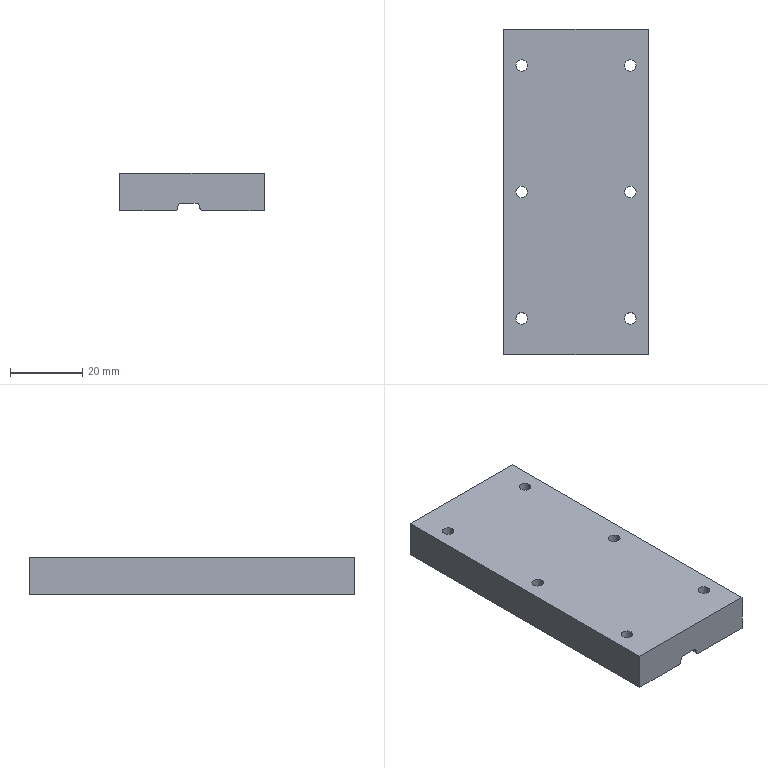Part | SolidWorks | features ICE 5, Extrusion 1, Fillet 1, MoveFace 1 | 1 solid | 26 faces | box 40 x 90 x 10.5 mm | volume 36117 mm3 | cylinder 16 | plane 10 | commonest cylinder face diameters 3.2 x12 2 x4
STEP:
#1=CARTESIAN_POINT('',(43.43,208.,0.5));
#2=VERTEX_POINT('',#1);
#3=CARTESIAN_POINT('',(46.63,208.,0.5));
#4=VERTEX_POINT('',#3);
#5=CARTESIAN_POINT('',(45.03,208.,0.5));
#6=DIRECTION('',(0.,0.,1.));
#7=DIRECTION('',(1.,0.,0.));
#8=AXIS2_PLACEMENT_3D('',#5,#6,#7);
#9=CIRCLE('',#8,1.6);
#10=EDGE_CURVE('',#2,#4,#9,.T.);
#11=ORIENTED_EDGE('',*,*,#10,.F.);
#12=CARTESIAN_POINT('',(43.43,208.,11.));
#13=VERTEX_POINT('',#12);
#14=CARTESIAN_POINT('',(43.43,208.,1.));
#15=DIRECTION('',(0.,0.,1.));
#16=VECTOR('',#15,1000.);
#17=LINE('',#14,#16);
#18=EDGE_CURVE('',#2,#13,#17,.T.);
#19=ORIENTED_EDGE('',*,*,#18,.T.);
#20=CARTESIAN_POINT('',(46.63,208.,11.));
#21=VERTEX_POINT('',#20);
#22=CARTESIAN_POINT('',(45.03,208.,11.));
#23=DIRECTION('',(0.,0.,1.));
#24=DIRECTION('',(1.,0.,0.));
#25=AXIS2_PLACEMENT_3D('',#22,#23,#24);
#26=CIRCLE('',#25,1.6);
#27=EDGE_CURVE('',#13,#21,#26,.T.);
#28=ORIENTED_EDGE('',*,*,#27,.T.);
#29=CARTESIAN_POINT('',(46.63,208.,1.));
#30=DIRECTION('',(0.,0.,1.));
#31=VECTOR('',#30,1000.);
#32=LINE('',#29,#31);
#33=EDGE_CURVE('',#4,#21,#32,.T.);
#34=ORIENTED_EDGE('',*,*,#33,.F.);
#35=EDGE_LOOP('',(#11,#19,#28,#34));
#36=FACE_OUTER_BOUND('',#35,.T.);
#37=CARTESIAN_POINT('',(45.03,208.,1.));
#38=DIRECTION('',(0.,0.,1.));
#39=DIRECTION('',(1.,0.,0.));
#40=AXIS2_PLACEMENT_3D('',#37,#38,#39);
#41=CYLINDRICAL_SURFACE('',#40,1.6);
#42=ADVANCED_FACE('',(#36),#41,.F.);
#43=CARTESIAN_POINT('',(43.43,173.,0.5));
#44=VERTEX_POINT('',#43);
#45=CARTESIAN_POINT('',(46.63,173.,0.5));
#46=VERTEX_POINT('',#45);
#47=CARTESIAN_POINT('',(45.03,173.,0.5));
#48=DIRECTION('',(0.,0.,1.));
#49=DIRECTION('',(1.,0.,0.));
#50=AXIS2_PLACEMENT_3D('',#47,#48,#49);
#51=CIRCLE('',#50,1.6);
#52=EDGE_CURVE('',#44,#46,#51,.T.);
#53=ORIENTED_EDGE('',*,*,#52,.F.);
#54=CARTESIAN_POINT('',(43.43,173.,11.));
#55=VERTEX_POINT('',#54);
#56=CARTESIAN_POINT('',(43.43,173.,1.));
#57=DIRECTION('',(0.,0.,1.));
#58=VECTOR('',#57,1000.);
#59=LINE('',#56,#58);
#60=EDGE_CURVE('',#44,#55,#59,.T.);
#61=ORIENTED_EDGE('',*,*,#60,.T.);
#62=CARTESIAN_POINT('',(46.63,173.,11.));
#63=VERTEX_POINT('',#62);
#64=CARTESIAN_POINT('',(45.03,173.,11.));
#65=DIRECTION('',(0.,0.,1.));
#66=DIRECTION('',(1.,0.,0.));
#67=AXIS2_PLACEMENT_3D('',#64,#65,#66);
#68=CIRCLE('',#67,1.6);
#69=EDGE_CURVE('',#55,#63,#68,.T.);
#70=ORIENTED_EDGE('',*,*,#69,.T.);
#71=CARTESIAN_POINT('',(46.63,173.,1.));
#72=DIRECTION('',(0.,0.,1.));
#73=VECTOR('',#72,1000.);
#74=LINE('',#71,#73);
#75=EDGE_CURVE('',#46,#63,#74,.T.);
#76=ORIENTED_EDGE('',*,*,#75,.F.);
#77=EDGE_LOOP('',(#53,#61,#70,#76));
#78=FACE_OUTER_BOUND('',#77,.T.);
#79=CARTESIAN_POINT('',(45.03,173.,1.));
#80=DIRECTION('',(0.,0.,1.));
#81=DIRECTION('',(1.,0.,0.));
#82=AXIS2_PLACEMENT_3D('',#79,#80,#81);
#83=CYLINDRICAL_SURFACE('',#82,1.6);
#84=ADVANCED_FACE('',(#78),#83,.F.);
#85=CARTESIAN_POINT('',(43.43,138.,0.5));
#86=VERTEX_POINT('',#85);
#87=CARTESIAN_POINT('',(46.63,138.,0.5));
#88=VERTEX_POINT('',#87);
#89=CARTESIAN_POINT('',(45.03,138.,0.5));
#90=DIRECTION('',(0.,0.,1.));
#91=DIRECTION('',(1.,0.,0.));
#92=AXIS2_PLACEMENT_3D('',#89,#90,#91);
#93=CIRCLE('',#92,1.6);
#94=EDGE_CURVE('',#86,#88,#93,.T.);
#95=ORIENTED_EDGE('',*,*,#94,.F.);
#96=CARTESIAN_POINT('',(43.43,138.,11.));
#97=VERTEX_POINT('',#96);
#98=CARTESIAN_POINT('',(43.43,138.,1.));
#99=DIRECTION('',(0.,0.,1.));
#100=VECTOR('',#99,1000.);
#101=LINE('',#98,#100);
#102=EDGE_CURVE('',#86,#97,#101,.T.);
#103=ORIENTED_EDGE('',*,*,#102,.T.);
#104=CARTESIAN_POINT('',(46.63,138.,11.));
#105=VERTEX_POINT('',#104);
#106=CARTESIAN_POINT('',(45.03,138.,11.));
#107=DIRECTION('',(0.,0.,1.));
#108=DIRECTION('',(1.,0.,0.));
#109=AXIS2_PLACEMENT_3D('',#106,#107,#108);
#110=CIRCLE('',#109,1.6);
#111=EDGE_CURVE('',#97,#105,#110,.T.);
#112=ORIENTED_EDGE('',*,*,#111,.T.);
#113=CARTESIAN_POINT('',(46.63,138.,1.));
#114=DIRECTION('',(0.,0.,1.));
#115=VECTOR('',#114,1000.);
#116=LINE('',#113,#115);
#117=EDGE_CURVE('',#88,#105,#116,.T.);
#118=ORIENTED_EDGE('',*,*,#117,.F.);
#119=EDGE_LOOP('',(#95,#103,#112,#118));
#120=FACE_OUTER_BOUND('',#119,.T.);
#121=CARTESIAN_POINT('',(45.03,138.,1.));
#122=DIRECTION('',(0.,0.,1.));
#123=DIRECTION('',(1.,0.,0.));
#124=AXIS2_PLACEMENT_3D('',#121,#122,#123);
#125=CYLINDRICAL_SURFACE('',#124,1.6);
#126=ADVANCED_FACE('',(#120),#125,.F.);
#127=CARTESIAN_POINT('',(13.37,173.,0.5));
#128=VERTEX_POINT('',#127);
#129=CARTESIAN_POINT('',(16.57,173.,0.5));
#130=VERTEX_POINT('',#129);
#131=CARTESIAN_POINT('',(14.97,173.,0.5));
#132=DIRECTION('',(0.,0.,1.));
#133=DIRECTION('',(1.,0.,0.));
#134=AXIS2_PLACEMENT_3D('',#131,#132,#133);
#135=CIRCLE('',#134,1.6);
#136=EDGE_CURVE('',#128,#130,#135,.T.);
#137=ORIENTED_EDGE('',*,*,#136,.F.);
#138=CARTESIAN_POINT('',(13.37,173.,11.));
#139=VERTEX_POINT('',#138);
#140=CARTESIAN_POINT('',(13.37,173.,1.));
#141=DIRECTION('',(0.,0.,1.));
#142=VECTOR('',#141,1000.);
#143=LINE('',#140,#142);
#144=EDGE_CURVE('',#128,#139,#143,.T.);
#145=ORIENTED_EDGE('',*,*,#144,.T.);
#146=CARTESIAN_POINT('',(16.57,173.,11.));
#147=VERTEX_POINT('',#146);
#148=CARTESIAN_POINT('',(14.97,173.,11.));
#149=DIRECTION('',(0.,0.,1.));
#150=DIRECTION('',(1.,0.,0.));
#151=AXIS2_PLACEMENT_3D('',#148,#149,#150);
#152=CIRCLE('',#151,1.6);
#153=EDGE_CURVE('',#139,#147,#152,.T.);
#154=ORIENTED_EDGE('',*,*,#153,.T.);
#155=CARTESIAN_POINT('',(16.57,173.,1.));
#156=DIRECTION('',(0.,0.,1.));
#157=VECTOR('',#156,1000.);
#158=LINE('',#155,#157);
#159=EDGE_CURVE('',#130,#147,#158,.T.);
#160=ORIENTED_EDGE('',*,*,#159,.F.);
#161=EDGE_LOOP('',(#137,#145,#154,#160));
#162=FACE_OUTER_BOUND('',#161,.T.);
#163=CARTESIAN_POINT('',(14.97,173.,1.));
#164=DIRECTION('',(0.,0.,1.));
#165=DIRECTION('',(1.,0.,0.));
#166=AXIS2_PLACEMENT_3D('',#163,#164,#165);
#167=CYLINDRICAL_SURFACE('',#166,1.6);
#168=ADVANCED_FACE('',(#162),#167,.F.);
#169=CARTESIAN_POINT('',(13.37,138.,0.5));
#170=VERTEX_POINT('',#169);
#171=CARTESIAN_POINT('',(16.57,138.,0.5));
#172=VERTEX_POINT('',#171);
#173=CARTESIAN_POINT('',(14.97,138.,0.5));
#174=DIRECTION('',(0.,0.,1.));
#175=DIRECTION('',(1.,0.,0.));
#176=AXIS2_PLACEMENT_3D('',#173,#174,#175);
#177=CIRCLE('',#176,1.6);
#178=EDGE_CURVE('',#170,#172,#177,.T.);
#179=ORIENTED_EDGE('',*,*,#178,.F.);
#180=CARTESIAN_POINT('',(13.37,138.,11.));
#181=VERTEX_POINT('',#180);
#182=CARTESIAN_POINT('',(13.37,138.,1.));
#183=DIRECTION('',(0.,0.,1.));
#184=VECTOR('',#183,1000.);
#185=LINE('',#182,#184);
#186=EDGE_CURVE('',#170,#181,#185,.T.);
#187=ORIENTED_EDGE('',*,*,#186,.T.);
#188=CARTESIAN_POINT('',(16.57,138.,11.));
#189=VERTEX_POINT('',#188);
#190=CARTESIAN_POINT('',(14.97,138.,11.));
#191=DIRECTION('',(0.,0.,1.));
#192=DIRECTION('',(1.,0.,0.));
#193=AXIS2_PLACEMENT_3D('',#190,#191,#192);
#194=CIRCLE('',#193,1.6);
#195=EDGE_CURVE('',#181,#189,#194,.T.);
#196=ORIENTED_EDGE('',*,*,#195,.T.);
#197=CARTESIAN_POINT('',(16.57,138.,1.));
#198=DIRECTION('',(0.,0.,1.));
#199=VECTOR('',#198,1000.);
#200=LINE('',#197,#199);
#201=EDGE_CURVE('',#172,#189,#200,.T.);
#202=ORIENTED_EDGE('',*,*,#201,.F.);
#203=EDGE_LOOP('',(#179,#187,#196,#202));
#204=FACE_OUTER_BOUND('',#203,.T.);
#205=CARTESIAN_POINT('',(14.97,138.,1.));
#206=DIRECTION('',(0.,0.,1.));
#207=DIRECTION('',(1.,0.,0.));
#208=AXIS2_PLACEMENT_3D('',#205,#206,#207);
#209=CYLINDRICAL_SURFACE('',#208,1.6);
#210=ADVANCED_FACE('',(#204),#209,.F.);
#211=CARTESIAN_POINT('',(13.37,208.,0.5));
#212=VERTEX_POINT('',#211);
#213=CARTESIAN_POINT('',(16.57,208.,0.5));
#214=VERTEX_POINT('',#213);
#215=CARTESIAN_POINT('',(14.97,208.,0.5));
#216=DIRECTION('',(0.,0.,1.));
#217=DIRECTION('',(1.,0.,0.));
#218=AXIS2_PLACEMENT_3D('',#215,#216,#217);
#219=CIRCLE('',#218,1.6);
#220=EDGE_CURVE('',#212,#214,#219,.T.);
#221=ORIENTED_EDGE('',*,*,#220,.F.);
#222=CARTESIAN_POINT('',(13.37,208.,11.));
#223=VERTEX_POINT('',#222);
#224=CARTESIAN_POINT('',(13.37,208.,1.));
#225=DIRECTION('',(0.,0.,1.));
#226=VECTOR('',#225,1000.);
#227=LINE('',#224,#226);
#228=EDGE_CURVE('',#212,#223,#227,.T.);
#229=ORIENTED_EDGE('',*,*,#228,.T.);
#230=CARTESIAN_POINT('',(16.57,208.,11.));
#231=VERTEX_POINT('',#230);
#232=CARTESIAN_POINT('',(14.97,208.,11.));
#233=DIRECTION('',(0.,0.,1.));
#234=DIRECTION('',(1.,0.,0.));
#235=AXIS2_PLACEMENT_3D('',#232,#233,#234);
#236=CIRCLE('',#235,1.6);
#237=EDGE_CURVE('',#223,#231,#236,.T.);
#238=ORIENTED_EDGE('',*,*,#237,.T.);
#239=CARTESIAN_POINT('',(16.57,208.,1.));
#240=DIRECTION('',(0.,0.,1.));
#241=VECTOR('',#240,1000.);
#242=LINE('',#239,#241);
#243=EDGE_CURVE('',#214,#231,#242,.T.);
#244=ORIENTED_EDGE('',*,*,#243,.F.);
#245=EDGE_LOOP('',(#221,#229,#238,#244));
#246=FACE_OUTER_BOUND('',#245,.T.);
#247=CARTESIAN_POINT('',(14.97,208.,1.));
#248=DIRECTION('',(0.,0.,1.));
#249=DIRECTION('',(1.,0.,0.));
#250=AXIS2_PLACEMENT_3D('',#247,#248,#249);
#251=CYLINDRICAL_SURFACE('',#250,1.6);
#252=ADVANCED_FACE('',(#246),#251,.F.);
#253=CARTESIAN_POINT('',(45.03,208.,0.5));
#254=DIRECTION('',(0.,0.,1.));
#255=DIRECTION('',(1.,0.,0.));
#256=AXIS2_PLACEMENT_3D('',#253,#254,#255);
#257=CIRCLE('',#256,1.6);
#258=EDGE_CURVE('',#4,#2,#257,.T.);
#259=ORIENTED_EDGE('',*,*,#258,.T.);
#260=ORIENTED_EDGE('',*,*,#10,.T.);
#261=EDGE_LOOP('',(#259,#260));
#262=FACE_BOUND('',#261,.T.);
#263=CARTESIAN_POINT('',(45.03,173.,0.5));
#264=DIRECTION('',(0.,0.,1.));
#265=DIRECTION('',(1.,0.,0.));
#266=AXIS2_PLACEMENT_3D('',#263,#264,#265);
#267=CIRCLE('',#266,1.6);
#268=EDGE_CURVE('',#46,#44,#267,.T.);
#269=ORIENTED_EDGE('',*,*,#268,.T.);
#270=ORIENTED_EDGE('',*,*,#52,.T.);
#271=EDGE_LOOP('',(#269,#270));
#272=FACE_BOUND('',#271,.T.);
#273=CARTESIAN_POINT('',(45.03,138.,0.5));
#274=DIRECTION('',(0.,0.,1.));
#275=DIRECTION('',(1.,0.,0.));
#276=AXIS2_PLACEMENT_3D('',#273,#274,#275);
#277=CIRCLE('',#276,1.6);
#278=EDGE_CURVE('',#88,#86,#277,.T.);
#279=ORIENTED_EDGE('',*,*,#278,.T.);
#280=ORIENTED_EDGE('',*,*,#94,.T.);
#281=EDGE_LOOP('',(#279,#280));
#282=FACE_BOUND('',#281,.T.);
#283=CARTESIAN_POINT('',(50.,128.,0.5));
#284=VERTEX_POINT('',#283);
#285=CARTESIAN_POINT('',(33.126,128.,0.5));
#286=VERTEX_POINT('',#285);
#287=CARTESIAN_POINT('',(10.,128.,0.5));
#288=DIRECTION('',(-1.,0.,0.));
#289=VECTOR('',#288,1000.);
#290=LINE('',#287,#289);
#291=EDGE_CURVE('',#284,#286,#290,.T.);
#292=ORIENTED_EDGE('',*,*,#291,.T.);
#293=CARTESIAN_POINT('',(33.126,218.,0.5));
#294=VERTEX_POINT('',#293);
#295=CARTESIAN_POINT('',(33.126,218.,0.5));
#296=DIRECTION('',(0.,1.,0.));
#297=VECTOR('',#296,1000.);
#298=LINE('',#295,#297);
#299=EDGE_CURVE('',#286,#294,#298,.T.);
#300=ORIENTED_EDGE('',*,*,#299,.T.);
#301=CARTESIAN_POINT('',(50.,218.,0.5));
#302=VERTEX_POINT('',#301);
#303=CARTESIAN_POINT('',(32.126,218.,0.5));
#304=DIRECTION('',(-1.,0.,0.));
#305=VECTOR('',#304,1000.);
#306=LINE('',#303,#305);
#307=EDGE_CURVE('',#302,#294,#306,.T.);
#308=ORIENTED_EDGE('',*,*,#307,.F.);
#309=CARTESIAN_POINT('',(50.,218.,0.5));
#310=DIRECTION('',(0.,-1.,0.));
#311=VECTOR('',#310,1000.);
#312=LINE('',#309,#311);
#313=EDGE_CURVE('',#302,#284,#312,.T.);
#314=ORIENTED_EDGE('',*,*,#313,.T.);
#315=EDGE_LOOP('',(#292,#300,#308,#314));
#316=FACE_OUTER_BOUND('',#315,.T.);
#317=CARTESIAN_POINT('',(32.126,218.,0.5));
#318=DIRECTION('',(0.,0.,1.));
#319=DIRECTION('',(1.,0.,0.));
#320=AXIS2_PLACEMENT_3D('',#317,#318,#319);
#321=PLANE('',#320);
#322=ADVANCED_FACE('',(#262,#272,#282,#316),#321,.F.);
#323=CARTESIAN_POINT('',(50.,218.,11.));
#324=VERTEX_POINT('',#323);
#325=CARTESIAN_POINT('',(50.,128.,11.));
#326=VERTEX_POINT('',#325);
#327=CARTESIAN_POINT('',(50.,218.,11.));
#328=DIRECTION('',(0.,-1.,0.));
#329=VECTOR('',#328,1000.);
#330=LINE('',#327,#329);
#331=EDGE_CURVE('',#324,#326,#330,.T.);
#332=ORIENTED_EDGE('',*,*,#331,.T.);
#333=CARTESIAN_POINT('',(50.,128.,1.));
#334=DIRECTION('',(0.,0.,1.));
#335=VECTOR('',#334,1000.);
#336=LINE('',#333,#335);
#337=EDGE_CURVE('',#284,#326,#336,.T.);
#338=ORIENTED_EDGE('',*,*,#337,.F.);
#339=ORIENTED_EDGE('',*,*,#313,.F.);
#340=CARTESIAN_POINT('',(50.,218.,1.));
#341=DIRECTION('',(0.,0.,-1.));
#342=VECTOR('',#341,1000.);
#343=LINE('',#340,#342);
#344=EDGE_CURVE('',#324,#302,#343,.T.);
#345=ORIENTED_EDGE('',*,*,#344,.F.);
#346=EDGE_LOOP('',(#332,#338,#339,#345));
#347=FACE_OUTER_BOUND('',#346,.T.);
#348=CARTESIAN_POINT('',(50.,50.,25.));
#349=DIRECTION('',(-1.,0.,0.));
#350=DIRECTION('',(0.,0.,1.));
#351=AXIS2_PLACEMENT_3D('',#348,#349,#350);
#352=PLANE('',#351);
#353=ADVANCED_FACE('',(#347),#352,.F.);
#354=CARTESIAN_POINT('',(10.,218.,0.5));
#355=VERTEX_POINT('',#354);
#356=CARTESIAN_POINT('',(10.,128.,0.5));
#357=VERTEX_POINT('',#356);
#358=CARTESIAN_POINT('',(10.,218.,0.5));
#359=DIRECTION('',(0.,-1.,0.));
#360=VECTOR('',#359,1000.);
#361=LINE('',#358,#360);
#362=EDGE_CURVE('',#355,#357,#361,.T.);
#363=ORIENTED_EDGE('',*,*,#362,.T.);
#364=CARTESIAN_POINT('',(10.,128.,11.));
#365=VERTEX_POINT('',#364);
#366=CARTESIAN_POINT('',(10.,128.,1.));
#367=DIRECTION('',(0.,0.,1.));
#368=VECTOR('',#367,1000.);
#369=LINE('',#366,#368);
#370=EDGE_CURVE('',#357,#365,#369,.T.);
#371=ORIENTED_EDGE('',*,*,#370,.T.);
#372=CARTESIAN_POINT('',(10.,218.,11.));
#373=VERTEX_POINT('',#372);
#374=CARTESIAN_POINT('',(10.,218.,11.));
#375=DIRECTION('',(0.,-1.,0.));
#376=VECTOR('',#375,1000.);
#377=LINE('',#374,#376);
#378=EDGE_CURVE('',#373,#365,#377,.T.);
#379=ORIENTED_EDGE('',*,*,#378,.F.);
#380=CARTESIAN_POINT('',(10.,218.,1.));
#381=DIRECTION('',(0.,0.,1.));
#382=VECTOR('',#381,1000.);
#383=LINE('',#380,#382);
#384=EDGE_CURVE('',#355,#373,#383,.T.);
#385=ORIENTED_EDGE('',*,*,#384,.F.);
#386=EDGE_LOOP('',(#363,#371,#379,#385));
#387=FACE_OUTER_BOUND('',#386,.T.);
#388=CARTESIAN_POINT('',(10.,218.,1.));
#389=DIRECTION('',(1.,0.,0.));
#390=DIRECTION('',(0.,0.,-1.));
#391=AXIS2_PLACEMENT_3D('',#388,#389,#390);
#392=PLANE('',#391);
#393=ADVANCED_FACE('',(#387),#392,.F.);
#394=CARTESIAN_POINT('',(14.97,173.,11.));
#395=DIRECTION('',(0.,0.,1.));
#396=DIRECTION('',(1.,0.,0.));
#397=AXIS2_PLACEMENT_3D('',#394,#395,#396);
#398=CIRCLE('',#397,1.6);
#399=EDGE_CURVE('',#147,#139,#398,.T.);
#400=ORIENTED_EDGE('',*,*,#399,.F.);
#401=ORIENTED_EDGE('',*,*,#153,.F.);
#402=EDGE_LOOP('',(#400,#401));
#403=FACE_BOUND('',#402,.T.);
#404=CARTESIAN_POINT('',(14.97,138.,11.));
#405=DIRECTION('',(0.,0.,1.));
#406=DIRECTION('',(1.,0.,0.));
#407=AXIS2_PLACEMENT_3D('',#404,#405,#406);
#408=CIRCLE('',#407,1.6);
#409=EDGE_CURVE('',#189,#181,#408,.T.);
#410=ORIENTED_EDGE('',*,*,#409,.F.);
#411=ORIENTED_EDGE('',*,*,#195,.F.);
#412=EDGE_LOOP('',(#410,#411));
#413=FACE_BOUND('',#412,.T.);
#414=CARTESIAN_POINT('',(45.03,208.,11.));
#415=DIRECTION('',(0.,0.,1.));
#416=DIRECTION('',(1.,0.,0.));
#417=AXIS2_PLACEMENT_3D('',#414,#415,#416);
#418=CIRCLE('',#417,1.6);
#419=EDGE_CURVE('',#21,#13,#418,.T.);
#420=ORIENTED_EDGE('',*,*,#419,.F.);
#421=ORIENTED_EDGE('',*,*,#27,.F.);
#422=EDGE_LOOP('',(#420,#421));
#423=FACE_BOUND('',#422,.T.);
#424=CARTESIAN_POINT('',(45.03,173.,11.));
#425=DIRECTION('',(0.,0.,1.));
#426=DIRECTION('',(1.,0.,0.));
#427=AXIS2_PLACEMENT_3D('',#424,#425,#426);
#428=CIRCLE('',#427,1.6);
#429=EDGE_CURVE('',#63,#55,#428,.T.);
#430=ORIENTED_EDGE('',*,*,#429,.F.);
#431=ORIENTED_EDGE('',*,*,#69,.F.);
#432=EDGE_LOOP('',(#430,#431));
#433=FACE_BOUND('',#432,.T.);
#434=CARTESIAN_POINT('',(45.03,138.,11.));
#435=DIRECTION('',(0.,0.,1.));
#436=DIRECTION('',(1.,0.,0.));
#437=AXIS2_PLACEMENT_3D('',#434,#435,#436);
#438=CIRCLE('',#437,1.6);
#439=EDGE_CURVE('',#105,#97,#438,.T.);
#440=ORIENTED_EDGE('',*,*,#439,.F.);
#441=ORIENTED_EDGE('',*,*,#111,.F.);
#442=EDGE_LOOP('',(#440,#441));
#443=FACE_BOUND('',#442,.T.);
#444=CARTESIAN_POINT('',(14.97,208.,11.));
#445=DIRECTION('',(0.,0.,1.));
#446=DIRECTION('',(1.,0.,0.));
#447=AXIS2_PLACEMENT_3D('',#444,#445,#446);
#448=CIRCLE('',#447,1.6);
#449=EDGE_CURVE('',#231,#223,#448,.T.);
#450=ORIENTED_EDGE('',*,*,#449,.F.);
#451=ORIENTED_EDGE('',*,*,#237,.F.);
#452=EDGE_LOOP('',(#450,#451));
#453=FACE_BOUND('',#452,.T.);
#454=ORIENTED_EDGE('',*,*,#378,.T.);
#455=CARTESIAN_POINT('',(10.,128.,11.));
#456=DIRECTION('',(-1.,0.,0.));
#457=VECTOR('',#456,1000.);
#458=LINE('',#455,#457);
#459=EDGE_CURVE('',#326,#365,#458,.T.);
#460=ORIENTED_EDGE('',*,*,#459,.F.);
#461=ORIENTED_EDGE('',*,*,#331,.F.);
#462=CARTESIAN_POINT('',(10.,218.,11.));
#463=DIRECTION('',(1.,0.,0.));
#464=VECTOR('',#463,1000.);
#465=LINE('',#462,#464);
#466=EDGE_CURVE('',#373,#324,#465,.T.);
#467=ORIENTED_EDGE('',*,*,#466,.F.);
#468=EDGE_LOOP('',(#454,#460,#461,#467));
#469=FACE_OUTER_BOUND('',#468,.T.);
#470=CARTESIAN_POINT('',(10.,218.,11.));
#471=DIRECTION('',(0.,0.,-1.));
#472=DIRECTION('',(-1.,0.,0.));
#473=AXIS2_PLACEMENT_3D('',#470,#471,#472);
#474=PLANE('',#473);
#475=ADVANCED_FACE('',(#403,#413,#423,#433,#443,#453,#469),#474,.F.);
#476=CARTESIAN_POINT('',(14.97,173.,0.5));
#477=DIRECTION('',(0.,0.,1.));
#478=DIRECTION('',(1.,0.,0.));
#479=AXIS2_PLACEMENT_3D('',#476,#477,#478);
#480=CIRCLE('',#479,1.6);
#481=EDGE_CURVE('',#130,#128,#480,.T.);
#482=ORIENTED_EDGE('',*,*,#481,.T.);
#483=ORIENTED_EDGE('',*,*,#136,.T.);
#484=EDGE_LOOP('',(#482,#483));
#485=FACE_BOUND('',#484,.T.);
#486=CARTESIAN_POINT('',(14.97,138.,0.5));
#487=DIRECTION('',(0.,0.,1.));
#488=DIRECTION('',(1.,0.,0.));
#489=AXIS2_PLACEMENT_3D('',#486,#487,#488);
#490=CIRCLE('',#489,1.6);
#491=EDGE_CURVE('',#172,#170,#490,.T.);
#492=ORIENTED_EDGE('',*,*,#491,.T.);
#493=ORIENTED_EDGE('',*,*,#178,.T.);
#494=EDGE_LOOP('',(#492,#493));
#495=FACE_BOUND('',#494,.T.);
#496=CARTESIAN_POINT('',(14.97,208.,0.5));
#497=DIRECTION('',(0.,0.,1.));
#498=DIRECTION('',(1.,0.,0.));
#499=AXIS2_PLACEMENT_3D('',#496,#497,#498);
#500=CIRCLE('',#499,1.6);
#501=EDGE_CURVE('',#214,#212,#500,.T.);
#502=ORIENTED_EDGE('',*,*,#501,.T.);
#503=ORIENTED_EDGE('',*,*,#220,.T.);
#504=EDGE_LOOP('',(#502,#503));
#505=FACE_BOUND('',#504,.T.);
#506=CARTESIAN_POINT('',(25.103,218.,0.5));
#507=VERTEX_POINT('',#506);
#508=CARTESIAN_POINT('',(10.,218.,0.5));
#509=DIRECTION('',(-1.,0.,0.));
#510=VECTOR('',#509,1000.);
#511=LINE('',#508,#510);
#512=EDGE_CURVE('',#507,#355,#511,.T.);
#513=ORIENTED_EDGE('',*,*,#512,.F.);
#514=CARTESIAN_POINT('',(25.103,128.,0.5));
#515=VERTEX_POINT('',#514);
#516=CARTESIAN_POINT('',(25.103,218.,0.5));
#517=DIRECTION('',(0.,-1.,0.));
#518=VECTOR('',#517,1000.);
#519=LINE('',#516,#518);
#520=EDGE_CURVE('',#507,#515,#519,.T.);
#521=ORIENTED_EDGE('',*,*,#520,.T.);
#522=CARTESIAN_POINT('',(10.,128.,0.5));
#523=DIRECTION('',(-1.,0.,0.));
#524=VECTOR('',#523,1000.);
#525=LINE('',#522,#524);
#526=EDGE_CURVE('',#515,#357,#525,.T.);
#527=ORIENTED_EDGE('',*,*,#526,.T.);
#528=ORIENTED_EDGE('',*,*,#362,.F.);
#529=EDGE_LOOP('',(#513,#521,#527,#528));
#530=FACE_OUTER_BOUND('',#529,.T.);
#531=CARTESIAN_POINT('',(32.126,218.,0.5));
#532=DIRECTION('',(0.,0.,1.));
#533=DIRECTION('',(1.,0.,0.));
#534=AXIS2_PLACEMENT_3D('',#531,#532,#533);
#535=PLANE('',#534);
#536=ADVANCED_FACE('',(#485,#495,#505,#530),#535,.F.);
#537=CARTESIAN_POINT('',(32.126,128.,1.5));
#538=VERTEX_POINT('',#537);
#539=CARTESIAN_POINT('',(32.126,128.,1.67));
#540=VERTEX_POINT('',#539);
#541=CARTESIAN_POINT('',(32.126,128.,0.5));
#542=DIRECTION('',(0.,0.,1.));
#543=VECTOR('',#542,1000.);
#544=LINE('',#541,#543);
#545=EDGE_CURVE('',#538,#540,#544,.T.);
#546=ORIENTED_EDGE('',*,*,#545,.T.);
#547=CARTESIAN_POINT('',(32.126,218.,1.67));
#548=VERTEX_POINT('',#547);
#549=CARTESIAN_POINT('',(32.126,218.,1.67));
#550=DIRECTION('',(0.,1.,0.));
#551=VECTOR('',#550,1000.);
#552=LINE('',#549,#551);
#553=EDGE_CURVE('',#540,#548,#552,.T.);
#554=ORIENTED_EDGE('',*,*,#553,.T.);
#555=CARTESIAN_POINT('',(32.126,218.,1.5));
#556=VERTEX_POINT('',#555);
#557=CARTESIAN_POINT('',(32.126,218.,0.5));
#558=DIRECTION('',(0.,0.,1.));
#559=VECTOR('',#558,1000.);
#560=LINE('',#557,#559);
#561=EDGE_CURVE('',#556,#548,#560,.T.);
#562=ORIENTED_EDGE('',*,*,#561,.F.);
#563=CARTESIAN_POINT('',(32.126,218.,1.5));
#564=DIRECTION('',(0.,-1.,0.));
#565=VECTOR('',#564,1000.);
#566=LINE('',#563,#565);
#567=EDGE_CURVE('',#556,#538,#566,.T.);
#568=ORIENTED_EDGE('',*,*,#567,.T.);
#569=EDGE_LOOP('',(#546,#554,#562,#568));
#570=FACE_OUTER_BOUND('',#569,.T.);
#571=CARTESIAN_POINT('',(32.126,218.,0.5));
#572=DIRECTION('',(1.,0.,0.));
#573=DIRECTION('',(0.,0.,-1.));
#574=AXIS2_PLACEMENT_3D('',#571,#572,#573);
#575=PLANE('',#574);
#576=ADVANCED_FACE('',(#570),#575,.F.);
#577=CARTESIAN_POINT('',(31.126,128.,2.67));
#578=VERTEX_POINT('',#577);
#579=CARTESIAN_POINT('',(27.103,128.,2.67));
#580=VERTEX_POINT('',#579);
#581=CARTESIAN_POINT('',(26.103,128.,2.67));
#582=DIRECTION('',(-1.,0.,0.));
#583=VECTOR('',#582,1000.);
#584=LINE('',#581,#583);
#585=EDGE_CURVE('',#578,#580,#584,.T.);
#586=ORIENTED_EDGE('',*,*,#585,.T.);
#587=CARTESIAN_POINT('',(27.103,218.,2.67));
#588=VERTEX_POINT('',#587);
#589=CARTESIAN_POINT('',(27.103,218.,2.67));
#590=DIRECTION('',(0.,1.,0.));
#591=VECTOR('',#590,1000.);
#592=LINE('',#589,#591);
#593=EDGE_CURVE('',#580,#588,#592,.T.);
#594=ORIENTED_EDGE('',*,*,#593,.T.);
#595=CARTESIAN_POINT('',(31.126,218.,2.67));
#596=VERTEX_POINT('',#595);
#597=CARTESIAN_POINT('',(26.103,218.,2.67));
#598=DIRECTION('',(-1.,0.,0.));
#599=VECTOR('',#598,1000.);
#600=LINE('',#597,#599);
#601=EDGE_CURVE('',#596,#588,#600,.T.);
#602=ORIENTED_EDGE('',*,*,#601,.F.);
#603=CARTESIAN_POINT('',(31.126,128.,2.67));
#604=DIRECTION('',(0.,-1.,0.));
#605=VECTOR('',#604,1000.);
#606=LINE('',#603,#605);
#607=EDGE_CURVE('',#596,#578,#606,.T.);
#608=ORIENTED_EDGE('',*,*,#607,.T.);
#609=EDGE_LOOP('',(#586,#594,#602,#608));
#610=FACE_OUTER_BOUND('',#609,.T.);
#611=CARTESIAN_POINT('',(26.103,218.,2.67));
#612=DIRECTION('',(0.,0.,1.));
#613=DIRECTION('',(1.,0.,0.));
#614=AXIS2_PLACEMENT_3D('',#611,#612,#613);
#615=PLANE('',#614);
#616=ADVANCED_FACE('',(#610),#615,.F.);
#617=CARTESIAN_POINT('',(26.103,218.,1.67));
#618=VERTEX_POINT('',#617);
#619=CARTESIAN_POINT('',(26.103,218.,1.5));
#620=VERTEX_POINT('',#619);
#621=CARTESIAN_POINT('',(26.103,218.,0.5));
#622=DIRECTION('',(0.,0.,-1.));
#623=VECTOR('',#622,1000.);
#624=LINE('',#621,#623);
#625=EDGE_CURVE('',#618,#620,#624,.T.);
#626=ORIENTED_EDGE('',*,*,#625,.F.);
#627=CARTESIAN_POINT('',(26.103,128.,1.67));
#628=VERTEX_POINT('',#627);
#629=CARTESIAN_POINT('',(26.103,128.,1.67));
#630=DIRECTION('',(0.,-1.,0.));
#631=VECTOR('',#630,1000.);
#632=LINE('',#629,#631);
#633=EDGE_CURVE('',#618,#628,#632,.T.);
#634=ORIENTED_EDGE('',*,*,#633,.T.);
#635=CARTESIAN_POINT('',(26.103,128.,1.5));
#636=VERTEX_POINT('',#635);
#637=CARTESIAN_POINT('',(26.103,128.,0.5));
#638=DIRECTION('',(0.,0.,-1.));
#639=VECTOR('',#638,1000.);
#640=LINE('',#637,#639);
#641=EDGE_CURVE('',#628,#636,#640,.T.);
#642=ORIENTED_EDGE('',*,*,#641,.T.);
#643=CARTESIAN_POINT('',(26.103,218.,1.5));
#644=DIRECTION('',(0.,1.,0.));
#645=VECTOR('',#644,1000.);
#646=LINE('',#643,#645);
#647=EDGE_CURVE('',#636,#620,#646,.T.);
#648=ORIENTED_EDGE('',*,*,#647,.T.);
#649=EDGE_LOOP('',(#626,#634,#642,#648));
#650=FACE_OUTER_BOUND('',#649,.T.);
#651=CARTESIAN_POINT('',(26.103,218.,0.5));
#652=DIRECTION('',(-1.,0.,0.));
#653=DIRECTION('',(0.,0.,1.));
#654=AXIS2_PLACEMENT_3D('',#651,#652,#653);
#655=PLANE('',#654);
#656=ADVANCED_FACE('',(#650),#655,.F.);
#657=ORIENTED_EDGE('',*,*,#625,.T.);
#658=CARTESIAN_POINT('',(25.103,218.,1.5));
#659=DIRECTION('',(0.,1.,0.));
#660=DIRECTION('',(0.,0.,1.));
#661=AXIS2_PLACEMENT_3D('',#658,#659,#660);
#662=CIRCLE('',#661,1.);
#663=EDGE_CURVE('',#620,#507,#662,.T.);
#664=ORIENTED_EDGE('',*,*,#663,.T.);
#665=ORIENTED_EDGE('',*,*,#512,.T.);
#666=ORIENTED_EDGE('',*,*,#384,.T.);
#667=ORIENTED_EDGE('',*,*,#466,.T.);
#668=ORIENTED_EDGE('',*,*,#344,.T.);
#669=ORIENTED_EDGE('',*,*,#307,.T.);
#670=CARTESIAN_POINT('',(33.126,218.,1.5));
#671=DIRECTION('',(0.,1.,0.));
#672=DIRECTION('',(0.,0.,1.));
#673=AXIS2_PLACEMENT_3D('',#670,#671,#672);
#674=CIRCLE('',#673,1.);
#675=EDGE_CURVE('',#294,#556,#674,.T.);
#676=ORIENTED_EDGE('',*,*,#675,.T.);
#677=ORIENTED_EDGE('',*,*,#561,.T.);
#678=CARTESIAN_POINT('',(31.126,218.,1.67));
#679=DIRECTION('',(0.,-1.,0.));
#680=DIRECTION('',(0.,0.,1.));
#681=AXIS2_PLACEMENT_3D('',#678,#679,#680);
#682=CIRCLE('',#681,1.);
#683=EDGE_CURVE('',#548,#596,#682,.T.);
#684=ORIENTED_EDGE('',*,*,#683,.T.);
#685=ORIENTED_EDGE('',*,*,#601,.T.);
#686=CARTESIAN_POINT('',(27.103,218.,1.67));
#687=DIRECTION('',(0.,-1.,0.));
#688=DIRECTION('',(0.,0.,1.));
#689=AXIS2_PLACEMENT_3D('',#686,#687,#688);
#690=CIRCLE('',#689,1.);
#691=EDGE_CURVE('',#588,#618,#690,.T.);
#692=ORIENTED_EDGE('',*,*,#691,.T.);
#693=EDGE_LOOP('',(#657,#664,#665,#666,#667,#668,#669,#676,#677,#684,#685,#692));
#694=FACE_OUTER_BOUND('',#693,.T.);
#695=CARTESIAN_POINT('',(0.,218.,0.));
#696=DIRECTION('',(0.,1.,0.));
#697=DIRECTION('',(0.,0.,1.));
#698=AXIS2_PLACEMENT_3D('',#695,#696,#697);
#699=PLANE('',#698);
#700=ADVANCED_FACE('',(#694),#699,.T.);
#701=ORIENTED_EDGE('',*,*,#526,.F.);
#702=CARTESIAN_POINT('',(25.103,128.,1.5));
#703=DIRECTION('',(0.,-1.,0.));
#704=DIRECTION('',(0.,0.,1.));
#705=AXIS2_PLACEMENT_3D('',#702,#703,#704);
#706=CIRCLE('',#705,1.);
#707=EDGE_CURVE('',#515,#636,#706,.T.);
#708=ORIENTED_EDGE('',*,*,#707,.T.);
#709=ORIENTED_EDGE('',*,*,#641,.F.);
#710=CARTESIAN_POINT('',(27.103,128.,1.67));
#711=DIRECTION('',(0.,1.,0.));
#712=DIRECTION('',(0.,0.,1.));
#713=AXIS2_PLACEMENT_3D('',#710,#711,#712);
#714=CIRCLE('',#713,1.);
#715=EDGE_CURVE('',#628,#580,#714,.T.);
#716=ORIENTED_EDGE('',*,*,#715,.T.);
#717=ORIENTED_EDGE('',*,*,#585,.F.);
#718=CARTESIAN_POINT('',(31.126,128.,1.67));
#719=DIRECTION('',(0.,1.,0.));
#720=DIRECTION('',(0.,0.,1.));
#721=AXIS2_PLACEMENT_3D('',#718,#719,#720);
#722=CIRCLE('',#721,1.);
#723=EDGE_CURVE('',#578,#540,#722,.T.);
#724=ORIENTED_EDGE('',*,*,#723,.T.);
#725=ORIENTED_EDGE('',*,*,#545,.F.);
#726=CARTESIAN_POINT('',(33.126,128.,1.5));
#727=DIRECTION('',(0.,-1.,0.));
#728=DIRECTION('',(0.,0.,1.));
#729=AXIS2_PLACEMENT_3D('',#726,#727,#728);
#730=CIRCLE('',#729,1.);
#731=EDGE_CURVE('',#538,#286,#730,.T.);
#732=ORIENTED_EDGE('',*,*,#731,.T.);
#733=ORIENTED_EDGE('',*,*,#291,.F.);
#734=ORIENTED_EDGE('',*,*,#337,.T.);
#735=ORIENTED_EDGE('',*,*,#459,.T.);
#736=ORIENTED_EDGE('',*,*,#370,.F.);
#737=EDGE_LOOP('',(#701,#708,#709,#716,#717,#724,#725,#732,#733,#734,#735,#736));
#738=FACE_OUTER_BOUND('',#737,.T.);
#739=CARTESIAN_POINT('',(10.,128.,1.));
#740=DIRECTION('',(0.,1.,0.));
#741=DIRECTION('',(0.,0.,1.));
#742=AXIS2_PLACEMENT_3D('',#739,#740,#741);
#743=PLANE('',#742);
#744=ADVANCED_FACE('',(#738),#743,.F.);
#745=ORIENTED_EDGE('',*,*,#691,.F.);
#746=ORIENTED_EDGE('',*,*,#593,.F.);
#747=ORIENTED_EDGE('',*,*,#715,.F.);
#748=ORIENTED_EDGE('',*,*,#633,.F.);
#749=EDGE_LOOP('',(#745,#746,#747,#748));
#750=FACE_OUTER_BOUND('',#749,.T.);
#751=CARTESIAN_POINT('',(27.103,218.,1.67));
#752=DIRECTION('',(0.,1.,0.));
#753=DIRECTION('',(0.,0.,1.));
#754=AXIS2_PLACEMENT_3D('',#751,#752,#753);
#755=CYLINDRICAL_SURFACE('',#754,1.);
#756=ADVANCED_FACE('',(#750),#755,.F.);
#757=ORIENTED_EDGE('',*,*,#683,.F.);
#758=ORIENTED_EDGE('',*,*,#553,.F.);
#759=ORIENTED_EDGE('',*,*,#723,.F.);
#760=ORIENTED_EDGE('',*,*,#607,.F.);
#761=EDGE_LOOP('',(#757,#758,#759,#760));
#762=FACE_OUTER_BOUND('',#761,.T.);
#763=CARTESIAN_POINT('',(31.126,218.,1.67));
#764=DIRECTION('',(0.,1.,0.));
#765=DIRECTION('',(0.,0.,1.));
#766=AXIS2_PLACEMENT_3D('',#763,#764,#765);
#767=CYLINDRICAL_SURFACE('',#766,1.);
#768=ADVANCED_FACE('',(#762),#767,.F.);
#769=ORIENTED_EDGE('',*,*,#663,.F.);
#770=ORIENTED_EDGE('',*,*,#647,.F.);
#771=ORIENTED_EDGE('',*,*,#707,.F.);
#772=ORIENTED_EDGE('',*,*,#520,.F.);
#773=EDGE_LOOP('',(#769,#770,#771,#772));
#774=FACE_OUTER_BOUND('',#773,.T.);
#775=CARTESIAN_POINT('',(25.103,218.,1.5));
#776=DIRECTION('',(0.,-1.,0.));
#777=DIRECTION('',(0.,0.,-1.));
#778=AXIS2_PLACEMENT_3D('',#775,#776,#777);
#779=CYLINDRICAL_SURFACE('',#778,1.);
#780=ADVANCED_FACE('',(#774),#779,.T.);
#781=ORIENTED_EDGE('',*,*,#675,.F.);
#782=ORIENTED_EDGE('',*,*,#299,.F.);
#783=ORIENTED_EDGE('',*,*,#731,.F.);
#784=ORIENTED_EDGE('',*,*,#567,.F.);
#785=EDGE_LOOP('',(#781,#782,#783,#784));
#786=FACE_OUTER_BOUND('',#785,.T.);
#787=CARTESIAN_POINT('',(33.126,218.,1.5));
#788=DIRECTION('',(0.,-1.,0.));
#789=DIRECTION('',(0.,0.,-1.));
#790=AXIS2_PLACEMENT_3D('',#787,#788,#789);
#791=CYLINDRICAL_SURFACE('',#790,1.);
#792=ADVANCED_FACE('',(#786),#791,.T.);
#793=ORIENTED_EDGE('',*,*,#228,.F.);
#794=ORIENTED_EDGE('',*,*,#501,.F.);
#795=ORIENTED_EDGE('',*,*,#243,.T.);
#796=ORIENTED_EDGE('',*,*,#449,.T.);
#797=EDGE_LOOP('',(#793,#794,#795,#796));
#798=FACE_OUTER_BOUND('',#797,.T.);
#799=CARTESIAN_POINT('',(14.97,208.,1.));
#800=DIRECTION('',(0.,0.,1.));
#801=DIRECTION('',(1.,0.,0.));
#802=AXIS2_PLACEMENT_3D('',#799,#800,#801);
#803=CYLINDRICAL_SURFACE('',#802,1.6);
#804=ADVANCED_FACE('',(#798),#803,.F.);
#805=ORIENTED_EDGE('',*,*,#186,.F.);
#806=ORIENTED_EDGE('',*,*,#491,.F.);
#807=ORIENTED_EDGE('',*,*,#201,.T.);
#808=ORIENTED_EDGE('',*,*,#409,.T.);
#809=EDGE_LOOP('',(#805,#806,#807,#808));
#810=FACE_OUTER_BOUND('',#809,.T.);
#811=CARTESIAN_POINT('',(14.97,138.,1.));
#812=DIRECTION('',(0.,0.,1.));
#813=DIRECTION('',(1.,0.,0.));
#814=AXIS2_PLACEMENT_3D('',#811,#812,#813);
#815=CYLINDRICAL_SURFACE('',#814,1.6);
#816=ADVANCED_FACE('',(#810),#815,.F.);
#817=ORIENTED_EDGE('',*,*,#144,.F.);
#818=ORIENTED_EDGE('',*,*,#481,.F.);
#819=ORIENTED_EDGE('',*,*,#159,.T.);
#820=ORIENTED_EDGE('',*,*,#399,.T.);
#821=EDGE_LOOP('',(#817,#818,#819,#820));
#822=FACE_OUTER_BOUND('',#821,.T.);
#823=CARTESIAN_POINT('',(14.97,173.,1.));
#824=DIRECTION('',(0.,0.,1.));
#825=DIRECTION('',(1.,0.,0.));
#826=AXIS2_PLACEMENT_3D('',#823,#824,#825);
#827=CYLINDRICAL_SURFACE('',#826,1.6);
#828=ADVANCED_FACE('',(#822),#827,.F.);
#829=ORIENTED_EDGE('',*,*,#102,.F.);
#830=ORIENTED_EDGE('',*,*,#278,.F.);
#831=ORIENTED_EDGE('',*,*,#117,.T.);
#832=ORIENTED_EDGE('',*,*,#439,.T.);
#833=EDGE_LOOP('',(#829,#830,#831,#832));
#834=FACE_OUTER_BOUND('',#833,.T.);
#835=CARTESIAN_POINT('',(45.03,138.,1.));
#836=DIRECTION('',(0.,0.,1.));
#837=DIRECTION('',(1.,0.,0.));
#838=AXIS2_PLACEMENT_3D('',#835,#836,#837);
#839=CYLINDRICAL_SURFACE('',#838,1.6);
#840=ADVANCED_FACE('',(#834),#839,.F.);
#841=ORIENTED_EDGE('',*,*,#60,.F.);
#842=ORIENTED_EDGE('',*,*,#268,.F.);
#843=ORIENTED_EDGE('',*,*,#75,.T.);
#844=ORIENTED_EDGE('',*,*,#429,.T.);
#845=EDGE_LOOP('',(#841,#842,#843,#844));
#846=FACE_OUTER_BOUND('',#845,.T.);
#847=CARTESIAN_POINT('',(45.03,173.,1.));
#848=DIRECTION('',(0.,0.,1.));
#849=DIRECTION('',(1.,0.,0.));
#850=AXIS2_PLACEMENT_3D('',#847,#848,#849);
#851=CYLINDRICAL_SURFACE('',#850,1.6);
#852=ADVANCED_FACE('',(#846),#851,.F.);
#853=ORIENTED_EDGE('',*,*,#18,.F.);
#854=ORIENTED_EDGE('',*,*,#258,.F.);
#855=ORIENTED_EDGE('',*,*,#33,.T.);
#856=ORIENTED_EDGE('',*,*,#419,.T.);
#857=EDGE_LOOP('',(#853,#854,#855,#856));
#858=FACE_OUTER_BOUND('',#857,.T.);
#859=CARTESIAN_POINT('',(45.03,208.,1.));
#860=DIRECTION('',(0.,0.,1.));
#861=DIRECTION('',(1.,0.,0.));
#862=AXIS2_PLACEMENT_3D('',#859,#860,#861);
#863=CYLINDRICAL_SURFACE('',#862,1.6);
#864=ADVANCED_FACE('',(#858),#863,.F.);
#865=CLOSED_SHELL('',(#42,#84,#126,#168,#210,#252,#322,#353,#393,#475,#536,#576,#616,#656,#700,#744,#756,#768,#780,#792,#804,#816,#828,#840,#852,#864));
#866=MANIFOLD_SOLID_BREP('',#865);
#867=CARTESIAN_POINT('',(0.,0.,0.));
#868=DIRECTION('',(0.,0.,1.));
#869=DIRECTION('',(1.,0.,0.));
#870=AXIS2_PLACEMENT_3D('',#867,#868,#869);
#871=(LENGTH_UNIT()NAMED_UNIT(*)SI_UNIT(.MILLI.,.METRE.));
#872=UNCERTAINTY_MEASURE_WITH_UNIT(LENGTH_MEASURE(0.00001),#871,'','');
#873=(NAMED_UNIT(*)PLANE_ANGLE_UNIT()SI_UNIT($,.RADIAN.));
#874=(NAMED_UNIT(*)SI_UNIT($,.STERADIAN.)SOLID_ANGLE_UNIT());
#875=(GEOMETRIC_REPRESENTATION_CONTEXT(3)GLOBAL_UNCERTAINTY_ASSIGNED_CONTEXT((#872))GLOBAL_UNIT_ASSIGNED_CONTEXT((#871,#873,#874))REPRESENTATION_CONTEXT('',''));
#876=ADVANCED_BREP_SHAPE_REPRESENTATION('',(#866,#870),#875);